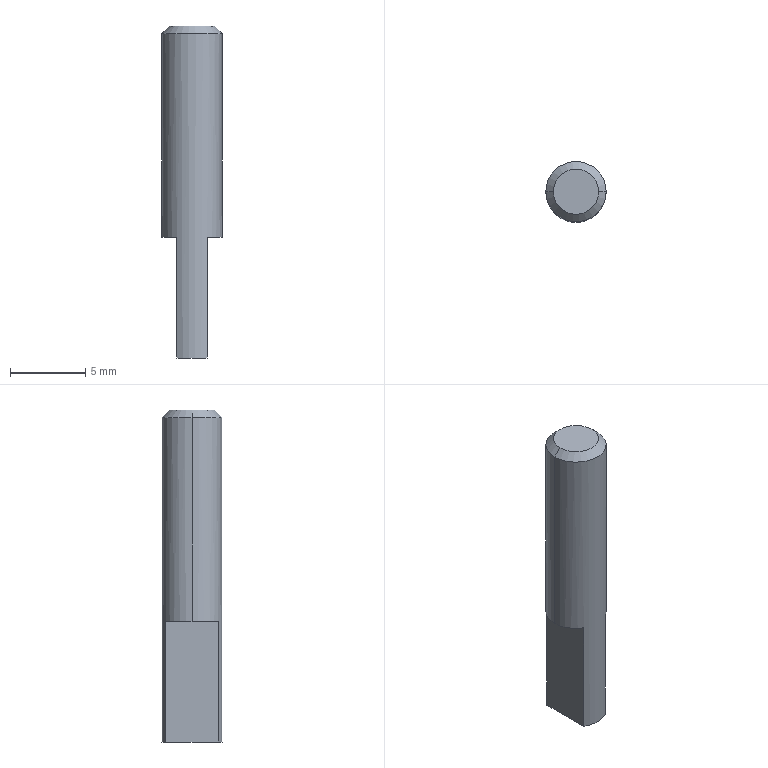Part | STEP file | PN_0104 Mount electronic clip sensor 2 | 1 solid | 10 faces | box 4 x 4 x 22 mm | volume 235.712 mm3 | plane 6 | cone 2 | cylinder 2 | commonest cylinder face diameters 4 x2
STEP:
#1=CARTESIAN_POINT('',(0.,0.,0.));
#2=DIRECTION('',(0.,0.,1.));
#3=DIRECTION('',(1.,0.,0.));
#4=AXIS2_PLACEMENT_3D('',#1,#2,#3);
#5=CARTESIAN_POINT('',(1.5,0.,22.));
#6=VERTEX_POINT('',#5);
#7=CARTESIAN_POINT('',(-1.5,0.,22.));
#8=VERTEX_POINT('',#7);
#9=CARTESIAN_POINT('',(0.,0.,22.));
#10=DIRECTION('',(0.,0.,1.));
#11=DIRECTION('',(1.,0.,0.));
#12=AXIS2_PLACEMENT_3D('',#9,#10,#11);
#13=CIRCLE('',#12,1.5);
#14=CARTESIAN_POINT('',(0.,0.,22.));
#15=DIRECTION('',(0.,0.,-1.));
#16=DIRECTION('',(-1.,0.,0.));
#17=AXIS2_PLACEMENT_3D('',#14,#15,#16);
#18=CONICAL_SURFACE('',#17,1.5,0.7854);
#19=CARTESIAN_POINT('',(3.142,0.));
#20=DIRECTION('',(-1.,0.));
#21=VECTOR('',#20,1.);
#22=LINE('',#19,#21);
#23=(GEOMETRIC_REPRESENTATION_CONTEXT(2)PARAMETRIC_REPRESENTATION_CONTEXT()REPRESENTATION_CONTEXT('',''));
#24=DEFINITIONAL_REPRESENTATION('',(#22),#23);
#25=PCURVE('',#18,#24);
#26=CARTESIAN_POINT('',(0.,0.,22.));
#27=DIRECTION('',(0.,0.,1.));
#28=DIRECTION('',(1.,0.,0.));
#29=AXIS2_PLACEMENT_3D('',#26,#27,#28);
#30=PLANE('',#29);
#31=CARTESIAN_POINT('',(0.,0.));
#32=DIRECTION('',(1.,0.));
#33=AXIS2_PLACEMENT_2D('',#31,#32);
#34=CIRCLE('',#33,1.5);
#35=(GEOMETRIC_REPRESENTATION_CONTEXT(2)PARAMETRIC_REPRESENTATION_CONTEXT()REPRESENTATION_CONTEXT('',''));
#36=DEFINITIONAL_REPRESENTATION('',(#34),#35);
#37=PCURVE('',#30,#36);
#38=SURFACE_CURVE('',#13,(#25,#37),.PCURVE_S1.);
#39=EDGE_CURVE('',#6,#8,#38,.T.);
#40=ORIENTED_EDGE('',*,*,#39,.F.);
#41=CARTESIAN_POINT('',(2.,0.,21.5));
#42=VERTEX_POINT('',#41);
#43=CARTESIAN_POINT('',(1.5,0.,22.));
#44=DIRECTION('',(0.7071,0.,-0.7071));
#45=VECTOR('',#44,1.);
#46=LINE('',#43,#45);
#47=CARTESIAN_POINT('',(3.142,0.));
#48=DIRECTION('',(0.,1.));
#49=VECTOR('',#48,1.);
#50=LINE('',#47,#49);
#51=(GEOMETRIC_REPRESENTATION_CONTEXT(2)PARAMETRIC_REPRESENTATION_CONTEXT()REPRESENTATION_CONTEXT('',''));
#52=DEFINITIONAL_REPRESENTATION('',(#50),#51);
#53=PCURVE('',#18,#52);
#54=CARTESIAN_POINT('',(0.,0.,22.));
#55=DIRECTION('',(0.,0.,-1.));
#56=DIRECTION('',(-1.,0.,0.));
#57=AXIS2_PLACEMENT_3D('',#54,#55,#56);
#58=CONICAL_SURFACE('',#57,1.5,0.7854);
#59=CARTESIAN_POINT('',(3.142,0.));
#60=DIRECTION('',(0.,1.));
#61=VECTOR('',#60,1.);
#62=LINE('',#59,#61);
#63=(GEOMETRIC_REPRESENTATION_CONTEXT(2)PARAMETRIC_REPRESENTATION_CONTEXT()REPRESENTATION_CONTEXT('',''));
#64=DEFINITIONAL_REPRESENTATION('',(#62),#63);
#65=PCURVE('',#58,#64);
#66=SURFACE_CURVE('',#46,(#53,#65),.PCURVE_S1.);
#67=EDGE_CURVE('',#6,#42,#66,.T.);
#68=ORIENTED_EDGE('',*,*,#67,.T.);
#69=CARTESIAN_POINT('',(-2.,0.,21.5));
#70=VERTEX_POINT('',#69);
#71=CARTESIAN_POINT('',(0.,0.,21.5));
#72=DIRECTION('',(0.,0.,-1.));
#73=DIRECTION('',(1.,0.,0.));
#74=AXIS2_PLACEMENT_3D('',#71,#72,#73);
#75=CIRCLE('',#74,2.);
#76=CARTESIAN_POINT('',(-3.142,0.5));
#77=DIRECTION('',(1.,0.));
#78=VECTOR('',#77,1.);
#79=LINE('',#76,#78);
#80=(GEOMETRIC_REPRESENTATION_CONTEXT(2)PARAMETRIC_REPRESENTATION_CONTEXT()REPRESENTATION_CONTEXT('',''));
#81=DEFINITIONAL_REPRESENTATION('',(#79),#80);
#82=PCURVE('',#18,#81);
#83=CARTESIAN_POINT('',(0.,0.,22.));
#84=DIRECTION('',(0.,0.,-1.));
#85=DIRECTION('',(-1.,0.,0.));
#86=AXIS2_PLACEMENT_3D('',#83,#84,#85);
#87=CYLINDRICAL_SURFACE('',#86,2.);
#88=CARTESIAN_POINT('',(-3.142,0.5));
#89=DIRECTION('',(1.,0.));
#90=VECTOR('',#89,1.);
#91=LINE('',#88,#90);
#92=(GEOMETRIC_REPRESENTATION_CONTEXT(2)PARAMETRIC_REPRESENTATION_CONTEXT()REPRESENTATION_CONTEXT('',''));
#93=DEFINITIONAL_REPRESENTATION('',(#91),#92);
#94=PCURVE('',#87,#93);
#95=SURFACE_CURVE('',#75,(#82,#94),.PCURVE_S1.);
#96=EDGE_CURVE('',#70,#42,#95,.T.);
#97=ORIENTED_EDGE('',*,*,#96,.F.);
#98=CARTESIAN_POINT('',(-1.5,0.,22.));
#99=DIRECTION('',(-0.7071,0.,-0.7071));
#100=VECTOR('',#99,1.);
#101=LINE('',#98,#100);
#102=CARTESIAN_POINT('',(0.,0.));
#103=DIRECTION('',(0.,1.));
#104=VECTOR('',#103,1.);
#105=LINE('',#102,#104);
#106=(GEOMETRIC_REPRESENTATION_CONTEXT(2)PARAMETRIC_REPRESENTATION_CONTEXT()REPRESENTATION_CONTEXT('',''));
#107=DEFINITIONAL_REPRESENTATION('',(#105),#106);
#108=PCURVE('',#18,#107);
#109=CARTESIAN_POINT('',(6.283,0.));
#110=DIRECTION('',(0.,1.));
#111=VECTOR('',#110,1.);
#112=LINE('',#109,#111);
#113=(GEOMETRIC_REPRESENTATION_CONTEXT(2)PARAMETRIC_REPRESENTATION_CONTEXT()REPRESENTATION_CONTEXT('',''));
#114=DEFINITIONAL_REPRESENTATION('',(#112),#113);
#115=PCURVE('',#58,#114);
#116=SURFACE_CURVE('',#101,(#108,#115),.PCURVE_S1.);
#117=EDGE_CURVE('',#8,#70,#116,.T.);
#118=ORIENTED_EDGE('',*,*,#117,.F.);
#119=EDGE_LOOP('',(#40,#68,#97,#118));
#120=FACE_BOUND('',#119,.T.);
#121=ADVANCED_FACE('',(#120),#18,.T.);
#122=ORIENTED_EDGE('',*,*,#96,.T.);
#123=CARTESIAN_POINT('',(2.,0.,8.));
#124=VERTEX_POINT('',#123);
#125=CARTESIAN_POINT('',(2.,0.,22.));
#126=DIRECTION('',(0.,0.,-1.));
#127=VECTOR('',#126,1.);
#128=LINE('',#125,#127);
#129=CARTESIAN_POINT('',(3.142,0.));
#130=DIRECTION('',(0.,1.));
#131=VECTOR('',#130,1.);
#132=LINE('',#129,#131);
#133=(GEOMETRIC_REPRESENTATION_CONTEXT(2)PARAMETRIC_REPRESENTATION_CONTEXT()REPRESENTATION_CONTEXT('',''));
#134=DEFINITIONAL_REPRESENTATION('',(#132),#133);
#135=PCURVE('',#87,#134);
#136=CARTESIAN_POINT('',(0.,0.,22.));
#137=DIRECTION('',(0.,0.,-1.));
#138=DIRECTION('',(-1.,0.,0.));
#139=AXIS2_PLACEMENT_3D('',#136,#137,#138);
#140=CYLINDRICAL_SURFACE('',#139,2.);
#141=CARTESIAN_POINT('',(3.142,0.));
#142=DIRECTION('',(0.,1.));
#143=VECTOR('',#142,1.);
#144=LINE('',#141,#143);
#145=(GEOMETRIC_REPRESENTATION_CONTEXT(2)PARAMETRIC_REPRESENTATION_CONTEXT()REPRESENTATION_CONTEXT('',''));
#146=DEFINITIONAL_REPRESENTATION('',(#144),#145);
#147=PCURVE('',#140,#146);
#148=SURFACE_CURVE('',#128,(#135,#147),.PCURVE_S1.);
#149=EDGE_CURVE('',#42,#124,#148,.T.);
#150=ORIENTED_EDGE('',*,*,#149,.T.);
#151=CARTESIAN_POINT('',(1.,1.732,8.));
#152=VERTEX_POINT('',#151);
#153=CARTESIAN_POINT('',(0.,0.,8.));
#154=DIRECTION('',(0.,0.,-1.));
#155=DIRECTION('',(-1.,0.,0.));
#156=AXIS2_PLACEMENT_3D('',#153,#154,#155);
#157=CIRCLE('',#156,2.);
#158=CARTESIAN_POINT('',(0.,14.));
#159=DIRECTION('',(1.,0.));
#160=VECTOR('',#159,1.);
#161=LINE('',#158,#160);
#162=(GEOMETRIC_REPRESENTATION_CONTEXT(2)PARAMETRIC_REPRESENTATION_CONTEXT()REPRESENTATION_CONTEXT('',''));
#163=DEFINITIONAL_REPRESENTATION('',(#161),#162);
#164=PCURVE('',#87,#163);
#165=CARTESIAN_POINT('',(0.,0.,8.));
#166=DIRECTION('',(0.,0.,-1.));
#167=DIRECTION('',(-1.,0.,0.));
#168=AXIS2_PLACEMENT_3D('',#165,#166,#167);
#169=PLANE('',#168);
#170=CARTESIAN_POINT('',(0.,0.));
#171=DIRECTION('',(1.,0.));
#172=AXIS2_PLACEMENT_2D('',#170,#171);
#173=CIRCLE('',#172,2.);
#174=(GEOMETRIC_REPRESENTATION_CONTEXT(2)PARAMETRIC_REPRESENTATION_CONTEXT()REPRESENTATION_CONTEXT('',''));
#175=DEFINITIONAL_REPRESENTATION('',(#173),#174);
#176=PCURVE('',#169,#175);
#177=SURFACE_CURVE('',#157,(#164,#176),.PCURVE_S1.);
#178=EDGE_CURVE('',#152,#124,#177,.T.);
#179=ORIENTED_EDGE('',*,*,#178,.F.);
#180=CARTESIAN_POINT('',(1.,1.732,0.));
#181=VERTEX_POINT('',#180);
#182=CARTESIAN_POINT('',(1.,1.732,22.));
#183=DIRECTION('',(0.,0.,-1.));
#184=VECTOR('',#183,1.);
#185=LINE('',#182,#184);
#186=CARTESIAN_POINT('',(2.094,0.));
#187=DIRECTION('',(0.,1.));
#188=VECTOR('',#187,1.);
#189=LINE('',#186,#188);
#190=(GEOMETRIC_REPRESENTATION_CONTEXT(2)PARAMETRIC_REPRESENTATION_CONTEXT()REPRESENTATION_CONTEXT('',''));
#191=DEFINITIONAL_REPRESENTATION('',(#189),#190);
#192=PCURVE('',#87,#191);
#193=CARTESIAN_POINT('',(1.,4.091,8.));
#194=DIRECTION('',(-1.,0.,0.));
#195=DIRECTION('',(0.,-1.,0.));
#196=AXIS2_PLACEMENT_3D('',#193,#194,#195);
#197=PLANE('',#196);
#198=CARTESIAN_POINT('',(2.359,14.));
#199=DIRECTION('',(0.,-1.));
#200=VECTOR('',#199,1.);
#201=LINE('',#198,#200);
#202=(GEOMETRIC_REPRESENTATION_CONTEXT(2)PARAMETRIC_REPRESENTATION_CONTEXT()REPRESENTATION_CONTEXT('',''));
#203=DEFINITIONAL_REPRESENTATION('',(#201),#202);
#204=PCURVE('',#197,#203);
#205=SURFACE_CURVE('',#185,(#192,#204),.PCURVE_S1.);
#206=EDGE_CURVE('',#152,#181,#205,.T.);
#207=ORIENTED_EDGE('',*,*,#206,.T.);
#208=CARTESIAN_POINT('',(-1.,1.732,0.));
#209=VERTEX_POINT('',#208);
#210=CARTESIAN_POINT('',(0.,0.,0.));
#211=DIRECTION('',(0.,0.,1.));
#212=DIRECTION('',(1.,0.,0.));
#213=AXIS2_PLACEMENT_3D('',#210,#211,#212);
#214=CIRCLE('',#213,2.);
#215=CARTESIAN_POINT('',(3.142,22.));
#216=DIRECTION('',(-1.,0.));
#217=VECTOR('',#216,1.);
#218=LINE('',#215,#217);
#219=(GEOMETRIC_REPRESENTATION_CONTEXT(2)PARAMETRIC_REPRESENTATION_CONTEXT()REPRESENTATION_CONTEXT('',''));
#220=DEFINITIONAL_REPRESENTATION('',(#218),#219);
#221=PCURVE('',#87,#220);
#222=CARTESIAN_POINT('',(0.,0.,0.));
#223=DIRECTION('',(0.,0.,1.));
#224=DIRECTION('',(1.,0.,0.));
#225=AXIS2_PLACEMENT_3D('',#222,#223,#224);
#226=PLANE('',#225);
#227=CARTESIAN_POINT('',(0.,0.));
#228=DIRECTION('',(1.,0.));
#229=AXIS2_PLACEMENT_2D('',#227,#228);
#230=CIRCLE('',#229,2.);
#231=(GEOMETRIC_REPRESENTATION_CONTEXT(2)PARAMETRIC_REPRESENTATION_CONTEXT()REPRESENTATION_CONTEXT('',''));
#232=DEFINITIONAL_REPRESENTATION('',(#230),#231);
#233=PCURVE('',#226,#232);
#234=SURFACE_CURVE('',#214,(#221,#233),.PCURVE_S1.);
#235=EDGE_CURVE('',#181,#209,#234,.T.);
#236=ORIENTED_EDGE('',*,*,#235,.T.);
#237=CARTESIAN_POINT('',(-1.,1.732,8.));
#238=VERTEX_POINT('',#237);
#239=CARTESIAN_POINT('',(-1.,1.732,22.));
#240=DIRECTION('',(0.,0.,1.));
#241=VECTOR('',#240,1.);
#242=LINE('',#239,#241);
#243=CARTESIAN_POINT('',(1.047,0.));
#244=DIRECTION('',(0.,-1.));
#245=VECTOR('',#244,1.);
#246=LINE('',#243,#245);
#247=(GEOMETRIC_REPRESENTATION_CONTEXT(2)PARAMETRIC_REPRESENTATION_CONTEXT()REPRESENTATION_CONTEXT('',''));
#248=DEFINITIONAL_REPRESENTATION('',(#246),#247);
#249=PCURVE('',#87,#248);
#250=CARTESIAN_POINT('',(-1.,3.929,8.));
#251=DIRECTION('',(1.,0.,0.));
#252=DIRECTION('',(0.,1.,0.));
#253=AXIS2_PLACEMENT_3D('',#250,#251,#252);
#254=PLANE('',#253);
#255=CARTESIAN_POINT('',(-2.197,14.));
#256=DIRECTION('',(0.,1.));
#257=VECTOR('',#256,1.);
#258=LINE('',#255,#257);
#259=(GEOMETRIC_REPRESENTATION_CONTEXT(2)PARAMETRIC_REPRESENTATION_CONTEXT()REPRESENTATION_CONTEXT('',''));
#260=DEFINITIONAL_REPRESENTATION('',(#258),#259);
#261=PCURVE('',#254,#260);
#262=SURFACE_CURVE('',#242,(#249,#261),.PCURVE_S1.);
#263=EDGE_CURVE('',#209,#238,#262,.T.);
#264=ORIENTED_EDGE('',*,*,#263,.T.);
#265=CARTESIAN_POINT('',(-2.,0.,8.));
#266=VERTEX_POINT('',#265);
#267=CARTESIAN_POINT('',(0.,0.,8.));
#268=DIRECTION('',(0.,0.,1.));
#269=DIRECTION('',(1.,0.,0.));
#270=AXIS2_PLACEMENT_3D('',#267,#268,#269);
#271=CIRCLE('',#270,2.);
#272=CARTESIAN_POINT('',(3.142,14.));
#273=DIRECTION('',(-1.,0.));
#274=VECTOR('',#273,1.);
#275=LINE('',#272,#274);
#276=(GEOMETRIC_REPRESENTATION_CONTEXT(2)PARAMETRIC_REPRESENTATION_CONTEXT()REPRESENTATION_CONTEXT('',''));
#277=DEFINITIONAL_REPRESENTATION('',(#275),#276);
#278=PCURVE('',#87,#277);
#279=CARTESIAN_POINT('',(0.,0.,8.));
#280=DIRECTION('',(0.,0.,1.));
#281=DIRECTION('',(1.,0.,0.));
#282=AXIS2_PLACEMENT_3D('',#279,#280,#281);
#283=PLANE('',#282);
#284=CARTESIAN_POINT('',(0.,0.));
#285=DIRECTION('',(1.,0.));
#286=AXIS2_PLACEMENT_2D('',#284,#285);
#287=CIRCLE('',#286,2.);
#288=(GEOMETRIC_REPRESENTATION_CONTEXT(2)PARAMETRIC_REPRESENTATION_CONTEXT()REPRESENTATION_CONTEXT('',''));
#289=DEFINITIONAL_REPRESENTATION('',(#287),#288);
#290=PCURVE('',#283,#289);
#291=SURFACE_CURVE('',#271,(#278,#290),.PCURVE_S1.);
#292=EDGE_CURVE('',#238,#266,#291,.T.);
#293=ORIENTED_EDGE('',*,*,#292,.T.);
#294=CARTESIAN_POINT('',(-2.,0.,22.));
#295=DIRECTION('',(0.,0.,-1.));
#296=VECTOR('',#295,1.);
#297=LINE('',#294,#296);
#298=CARTESIAN_POINT('',(0.,0.));
#299=DIRECTION('',(0.,1.));
#300=VECTOR('',#299,1.);
#301=LINE('',#298,#300);
#302=(GEOMETRIC_REPRESENTATION_CONTEXT(2)PARAMETRIC_REPRESENTATION_CONTEXT()REPRESENTATION_CONTEXT('',''));
#303=DEFINITIONAL_REPRESENTATION('',(#301),#302);
#304=PCURVE('',#87,#303);
#305=CARTESIAN_POINT('',(6.283,0.));
#306=DIRECTION('',(0.,1.));
#307=VECTOR('',#306,1.);
#308=LINE('',#305,#307);
#309=(GEOMETRIC_REPRESENTATION_CONTEXT(2)PARAMETRIC_REPRESENTATION_CONTEXT()REPRESENTATION_CONTEXT('',''));
#310=DEFINITIONAL_REPRESENTATION('',(#308),#309);
#311=PCURVE('',#140,#310);
#312=SURFACE_CURVE('',#297,(#304,#311),.PCURVE_S1.);
#313=EDGE_CURVE('',#70,#266,#312,.T.);
#314=ORIENTED_EDGE('',*,*,#313,.F.);
#315=EDGE_LOOP('',(#122,#150,#179,#207,#236,#264,#293,#314));
#316=FACE_BOUND('',#315,.T.);
#317=ADVANCED_FACE('',(#316),#87,.T.);
#318=ORIENTED_EDGE('',*,*,#149,.F.);
#319=CARTESIAN_POINT('',(0.,0.,21.5));
#320=DIRECTION('',(0.,0.,-1.));
#321=DIRECTION('',(1.,0.,0.));
#322=AXIS2_PLACEMENT_3D('',#319,#320,#321);
#323=CIRCLE('',#322,2.);
#324=CARTESIAN_POINT('',(3.142,0.5));
#325=DIRECTION('',(1.,0.));
#326=VECTOR('',#325,1.);
#327=LINE('',#324,#326);
#328=(GEOMETRIC_REPRESENTATION_CONTEXT(2)PARAMETRIC_REPRESENTATION_CONTEXT()REPRESENTATION_CONTEXT('',''));
#329=DEFINITIONAL_REPRESENTATION('',(#327),#328);
#330=PCURVE('',#140,#329);
#331=CARTESIAN_POINT('',(3.142,0.5));
#332=DIRECTION('',(1.,0.));
#333=VECTOR('',#332,1.);
#334=LINE('',#331,#333);
#335=(GEOMETRIC_REPRESENTATION_CONTEXT(2)PARAMETRIC_REPRESENTATION_CONTEXT()REPRESENTATION_CONTEXT('',''));
#336=DEFINITIONAL_REPRESENTATION('',(#334),#335);
#337=PCURVE('',#58,#336);
#338=SURFACE_CURVE('',#323,(#330,#337),.PCURVE_S1.);
#339=EDGE_CURVE('',#42,#70,#338,.T.);
#340=ORIENTED_EDGE('',*,*,#339,.T.);
#341=ORIENTED_EDGE('',*,*,#313,.T.);
#342=CARTESIAN_POINT('',(-1.,-1.732,8.));
#343=VERTEX_POINT('',#342);
#344=CARTESIAN_POINT('',(0.,0.,8.));
#345=DIRECTION('',(0.,0.,1.));
#346=DIRECTION('',(1.,0.,0.));
#347=AXIS2_PLACEMENT_3D('',#344,#345,#346);
#348=CIRCLE('',#347,2.);
#349=CARTESIAN_POINT('',(9.425,14.));
#350=DIRECTION('',(-1.,0.));
#351=VECTOR('',#350,1.);
#352=LINE('',#349,#351);
#353=(GEOMETRIC_REPRESENTATION_CONTEXT(2)PARAMETRIC_REPRESENTATION_CONTEXT()REPRESENTATION_CONTEXT('',''));
#354=DEFINITIONAL_REPRESENTATION('',(#352),#353);
#355=PCURVE('',#140,#354);
#356=CARTESIAN_POINT('',(0.,0.));
#357=DIRECTION('',(1.,0.));
#358=AXIS2_PLACEMENT_2D('',#356,#357);
#359=CIRCLE('',#358,2.);
#360=(GEOMETRIC_REPRESENTATION_CONTEXT(2)PARAMETRIC_REPRESENTATION_CONTEXT()REPRESENTATION_CONTEXT('',''));
#361=DEFINITIONAL_REPRESENTATION('',(#359),#360);
#362=PCURVE('',#283,#361);
#363=SURFACE_CURVE('',#348,(#355,#362),.PCURVE_S1.);
#364=EDGE_CURVE('',#266,#343,#363,.T.);
#365=ORIENTED_EDGE('',*,*,#364,.T.);
#366=CARTESIAN_POINT('',(-1.,-1.732,0.));
#367=VERTEX_POINT('',#366);
#368=CARTESIAN_POINT('',(-1.,-1.732,22.));
#369=DIRECTION('',(0.,0.,-1.));
#370=VECTOR('',#369,1.);
#371=LINE('',#368,#370);
#372=CARTESIAN_POINT('',(5.236,0.));
#373=DIRECTION('',(0.,1.));
#374=VECTOR('',#373,1.);
#375=LINE('',#372,#374);
#376=(GEOMETRIC_REPRESENTATION_CONTEXT(2)PARAMETRIC_REPRESENTATION_CONTEXT()REPRESENTATION_CONTEXT('',''));
#377=DEFINITIONAL_REPRESENTATION('',(#375),#376);
#378=PCURVE('',#140,#377);
#379=CARTESIAN_POINT('',(-5.661,14.));
#380=DIRECTION('',(0.,-1.));
#381=VECTOR('',#380,1.);
#382=LINE('',#379,#381);
#383=(GEOMETRIC_REPRESENTATION_CONTEXT(2)PARAMETRIC_REPRESENTATION_CONTEXT()REPRESENTATION_CONTEXT('',''));
#384=DEFINITIONAL_REPRESENTATION('',(#382),#383);
#385=PCURVE('',#254,#384);
#386=SURFACE_CURVE('',#371,(#378,#385),.PCURVE_S1.);
#387=EDGE_CURVE('',#343,#367,#386,.T.);
#388=ORIENTED_EDGE('',*,*,#387,.T.);
#389=CARTESIAN_POINT('',(1.,-1.732,0.));
#390=VERTEX_POINT('',#389);
#391=CARTESIAN_POINT('',(0.,0.,0.));
#392=DIRECTION('',(0.,0.,1.));
#393=DIRECTION('',(1.,0.,0.));
#394=AXIS2_PLACEMENT_3D('',#391,#392,#393);
#395=CIRCLE('',#394,2.);
#396=CARTESIAN_POINT('',(9.425,22.));
#397=DIRECTION('',(-1.,0.));
#398=VECTOR('',#397,1.);
#399=LINE('',#396,#398);
#400=(GEOMETRIC_REPRESENTATION_CONTEXT(2)PARAMETRIC_REPRESENTATION_CONTEXT()REPRESENTATION_CONTEXT('',''));
#401=DEFINITIONAL_REPRESENTATION('',(#399),#400);
#402=PCURVE('',#140,#401);
#403=CARTESIAN_POINT('',(0.,0.));
#404=DIRECTION('',(1.,0.));
#405=AXIS2_PLACEMENT_2D('',#403,#404);
#406=CIRCLE('',#405,2.);
#407=(GEOMETRIC_REPRESENTATION_CONTEXT(2)PARAMETRIC_REPRESENTATION_CONTEXT()REPRESENTATION_CONTEXT('',''));
#408=DEFINITIONAL_REPRESENTATION('',(#406),#407);
#409=PCURVE('',#226,#408);
#410=SURFACE_CURVE('',#395,(#402,#409),.PCURVE_S1.);
#411=EDGE_CURVE('',#367,#390,#410,.T.);
#412=ORIENTED_EDGE('',*,*,#411,.T.);
#413=CARTESIAN_POINT('',(1.,-1.732,8.));
#414=VERTEX_POINT('',#413);
#415=CARTESIAN_POINT('',(1.,-1.732,22.));
#416=DIRECTION('',(0.,0.,1.));
#417=VECTOR('',#416,1.);
#418=LINE('',#415,#417);
#419=CARTESIAN_POINT('',(4.189,0.));
#420=DIRECTION('',(0.,-1.));
#421=VECTOR('',#420,1.);
#422=LINE('',#419,#421);
#423=(GEOMETRIC_REPRESENTATION_CONTEXT(2)PARAMETRIC_REPRESENTATION_CONTEXT()REPRESENTATION_CONTEXT('',''));
#424=DEFINITIONAL_REPRESENTATION('',(#422),#423);
#425=PCURVE('',#140,#424);
#426=CARTESIAN_POINT('',(5.823,14.));
#427=DIRECTION('',(0.,1.));
#428=VECTOR('',#427,1.);
#429=LINE('',#426,#428);
#430=(GEOMETRIC_REPRESENTATION_CONTEXT(2)PARAMETRIC_REPRESENTATION_CONTEXT()REPRESENTATION_CONTEXT('',''));
#431=DEFINITIONAL_REPRESENTATION('',(#429),#430);
#432=PCURVE('',#197,#431);
#433=SURFACE_CURVE('',#418,(#425,#432),.PCURVE_S1.);
#434=EDGE_CURVE('',#390,#414,#433,.T.);
#435=ORIENTED_EDGE('',*,*,#434,.T.);
#436=CARTESIAN_POINT('',(0.,0.,8.));
#437=DIRECTION('',(0.,0.,-1.));
#438=DIRECTION('',(-1.,0.,0.));
#439=AXIS2_PLACEMENT_3D('',#436,#437,#438);
#440=CIRCLE('',#439,2.);
#441=CARTESIAN_POINT('',(0.,14.));
#442=DIRECTION('',(1.,0.));
#443=VECTOR('',#442,1.);
#444=LINE('',#441,#443);
#445=(GEOMETRIC_REPRESENTATION_CONTEXT(2)PARAMETRIC_REPRESENTATION_CONTEXT()REPRESENTATION_CONTEXT('',''));
#446=DEFINITIONAL_REPRESENTATION('',(#444),#445);
#447=PCURVE('',#140,#446);
#448=CARTESIAN_POINT('',(0.,0.));
#449=DIRECTION('',(1.,0.));
#450=AXIS2_PLACEMENT_2D('',#448,#449);
#451=CIRCLE('',#450,2.);
#452=(GEOMETRIC_REPRESENTATION_CONTEXT(2)PARAMETRIC_REPRESENTATION_CONTEXT()REPRESENTATION_CONTEXT('',''));
#453=DEFINITIONAL_REPRESENTATION('',(#451),#452);
#454=PCURVE('',#169,#453);
#455=SURFACE_CURVE('',#440,(#447,#454),.PCURVE_S1.);
#456=EDGE_CURVE('',#124,#414,#455,.T.);
#457=ORIENTED_EDGE('',*,*,#456,.F.);
#458=EDGE_LOOP('',(#318,#340,#341,#365,#388,#412,#435,#457));
#459=FACE_BOUND('',#458,.T.);
#460=ADVANCED_FACE('',(#459),#140,.T.);
#461=CARTESIAN_POINT('',(0.,0.,22.));
#462=DIRECTION('',(0.,0.,1.));
#463=DIRECTION('',(1.,0.,0.));
#464=AXIS2_PLACEMENT_3D('',#461,#462,#463);
#465=CIRCLE('',#464,1.5);
#466=CARTESIAN_POINT('',(0.,0.));
#467=DIRECTION('',(1.,0.));
#468=AXIS2_PLACEMENT_2D('',#466,#467);
#469=CIRCLE('',#468,1.5);
#470=(GEOMETRIC_REPRESENTATION_CONTEXT(2)PARAMETRIC_REPRESENTATION_CONTEXT()REPRESENTATION_CONTEXT('',''));
#471=DEFINITIONAL_REPRESENTATION('',(#469),#470);
#472=PCURVE('',#30,#471);
#473=CARTESIAN_POINT('',(9.425,0.));
#474=DIRECTION('',(-1.,0.));
#475=VECTOR('',#474,1.);
#476=LINE('',#473,#475);
#477=(GEOMETRIC_REPRESENTATION_CONTEXT(2)PARAMETRIC_REPRESENTATION_CONTEXT()REPRESENTATION_CONTEXT('',''));
#478=DEFINITIONAL_REPRESENTATION('',(#476),#477);
#479=PCURVE('',#58,#478);
#480=SURFACE_CURVE('',#465,(#472,#479),.PCURVE_S1.);
#481=EDGE_CURVE('',#8,#6,#480,.T.);
#482=ORIENTED_EDGE('',*,*,#481,.T.);
#483=ORIENTED_EDGE('',*,*,#39,.T.);
#484=EDGE_LOOP('',(#482,#483));
#485=FACE_BOUND('',#484,.T.);
#486=ADVANCED_FACE('',(#485),#30,.T.);
#487=ORIENTED_EDGE('',*,*,#411,.F.);
#488=CARTESIAN_POINT('',(-1.,0.,0.));
#489=DIRECTION('',(0.,1.,0.));
#490=VECTOR('',#489,1.);
#491=LINE('',#488,#490);
#492=CARTESIAN_POINT('',(-1.,0.));
#493=DIRECTION('',(0.,1.));
#494=VECTOR('',#493,1.);
#495=LINE('',#492,#494);
#496=(GEOMETRIC_REPRESENTATION_CONTEXT(2)PARAMETRIC_REPRESENTATION_CONTEXT()REPRESENTATION_CONTEXT('',''));
#497=DEFINITIONAL_REPRESENTATION('',(#495),#496);
#498=PCURVE('',#226,#497);
#499=CARTESIAN_POINT('',(-3.929,-8.));
#500=DIRECTION('',(1.,0.));
#501=VECTOR('',#500,1.);
#502=LINE('',#499,#501);
#503=(GEOMETRIC_REPRESENTATION_CONTEXT(2)PARAMETRIC_REPRESENTATION_CONTEXT()REPRESENTATION_CONTEXT('',''));
#504=DEFINITIONAL_REPRESENTATION('',(#502),#503);
#505=PCURVE('',#254,#504);
#506=SURFACE_CURVE('',#491,(#498,#505),.PCURVE_S1.);
#507=EDGE_CURVE('',#367,#209,#506,.T.);
#508=ORIENTED_EDGE('',*,*,#507,.T.);
#509=ORIENTED_EDGE('',*,*,#235,.F.);
#510=CARTESIAN_POINT('',(1.,0.,0.));
#511=DIRECTION('',(0.,-1.,0.));
#512=VECTOR('',#511,1.);
#513=LINE('',#510,#512);
#514=CARTESIAN_POINT('',(1.,0.));
#515=DIRECTION('',(0.,-1.));
#516=VECTOR('',#515,1.);
#517=LINE('',#514,#516);
#518=(GEOMETRIC_REPRESENTATION_CONTEXT(2)PARAMETRIC_REPRESENTATION_CONTEXT()REPRESENTATION_CONTEXT('',''));
#519=DEFINITIONAL_REPRESENTATION('',(#517),#518);
#520=PCURVE('',#226,#519);
#521=CARTESIAN_POINT('',(4.091,-8.));
#522=DIRECTION('',(1.,0.));
#523=VECTOR('',#522,1.);
#524=LINE('',#521,#523);
#525=(GEOMETRIC_REPRESENTATION_CONTEXT(2)PARAMETRIC_REPRESENTATION_CONTEXT()REPRESENTATION_CONTEXT('',''));
#526=DEFINITIONAL_REPRESENTATION('',(#524),#525);
#527=PCURVE('',#197,#526);
#528=SURFACE_CURVE('',#513,(#520,#527),.PCURVE_S1.);
#529=EDGE_CURVE('',#181,#390,#528,.T.);
#530=ORIENTED_EDGE('',*,*,#529,.T.);
#531=EDGE_LOOP('',(#487,#508,#509,#530));
#532=FACE_BOUND('',#531,.T.);
#533=ADVANCED_FACE('',(#532),#226,.F.);
#534=ORIENTED_EDGE('',*,*,#178,.T.);
#535=ORIENTED_EDGE('',*,*,#456,.T.);
#536=CARTESIAN_POINT('',(1.,4.091,8.));
#537=DIRECTION('',(0.,1.,0.));
#538=VECTOR('',#537,1.);
#539=LINE('',#536,#538);
#540=CARTESIAN_POINT('',(-1.,4.091));
#541=DIRECTION('',(0.,1.));
#542=VECTOR('',#541,1.);
#543=LINE('',#540,#542);
#544=(GEOMETRIC_REPRESENTATION_CONTEXT(2)PARAMETRIC_REPRESENTATION_CONTEXT()REPRESENTATION_CONTEXT('',''));
#545=DEFINITIONAL_REPRESENTATION('',(#543),#544);
#546=PCURVE('',#169,#545);
#547=CARTESIAN_POINT('',(0.,0.));
#548=DIRECTION('',(-1.,0.));
#549=VECTOR('',#548,1.);
#550=LINE('',#547,#549);
#551=(GEOMETRIC_REPRESENTATION_CONTEXT(2)PARAMETRIC_REPRESENTATION_CONTEXT()REPRESENTATION_CONTEXT('',''));
#552=DEFINITIONAL_REPRESENTATION('',(#550),#551);
#553=PCURVE('',#197,#552);
#554=SURFACE_CURVE('',#539,(#546,#553),.PCURVE_S1.);
#555=EDGE_CURVE('',#414,#152,#554,.T.);
#556=ORIENTED_EDGE('',*,*,#555,.T.);
#557=EDGE_LOOP('',(#534,#535,#556));
#558=FACE_BOUND('',#557,.T.);
#559=ADVANCED_FACE('',(#558),#169,.T.);
#560=ORIENTED_EDGE('',*,*,#555,.F.);
#561=ORIENTED_EDGE('',*,*,#434,.F.);
#562=ORIENTED_EDGE('',*,*,#529,.F.);
#563=ORIENTED_EDGE('',*,*,#206,.F.);
#564=EDGE_LOOP('',(#560,#561,#562,#563));
#565=FACE_BOUND('',#564,.T.);
#566=ADVANCED_FACE('',(#565),#197,.F.);
#567=CARTESIAN_POINT('',(-1.,3.929,8.));
#568=DIRECTION('',(0.,-1.,0.));
#569=VECTOR('',#568,1.);
#570=LINE('',#567,#569);
#571=CARTESIAN_POINT('',(-1.,3.929));
#572=DIRECTION('',(0.,-1.));
#573=VECTOR('',#572,1.);
#574=LINE('',#571,#573);
#575=(GEOMETRIC_REPRESENTATION_CONTEXT(2)PARAMETRIC_REPRESENTATION_CONTEXT()REPRESENTATION_CONTEXT('',''));
#576=DEFINITIONAL_REPRESENTATION('',(#574),#575);
#577=PCURVE('',#283,#576);
#578=CARTESIAN_POINT('',(0.,0.));
#579=DIRECTION('',(-1.,0.));
#580=VECTOR('',#579,1.);
#581=LINE('',#578,#580);
#582=(GEOMETRIC_REPRESENTATION_CONTEXT(2)PARAMETRIC_REPRESENTATION_CONTEXT()REPRESENTATION_CONTEXT('',''));
#583=DEFINITIONAL_REPRESENTATION('',(#581),#582);
#584=PCURVE('',#254,#583);
#585=SURFACE_CURVE('',#570,(#577,#584),.PCURVE_S1.);
#586=EDGE_CURVE('',#238,#343,#585,.T.);
#587=ORIENTED_EDGE('',*,*,#586,.T.);
#588=ORIENTED_EDGE('',*,*,#364,.F.);
#589=ORIENTED_EDGE('',*,*,#292,.F.);
#590=EDGE_LOOP('',(#587,#588,#589));
#591=FACE_BOUND('',#590,.T.);
#592=ADVANCED_FACE('',(#591),#283,.F.);
#593=ORIENTED_EDGE('',*,*,#586,.F.);
#594=ORIENTED_EDGE('',*,*,#263,.F.);
#595=ORIENTED_EDGE('',*,*,#507,.F.);
#596=ORIENTED_EDGE('',*,*,#387,.F.);
#597=EDGE_LOOP('',(#593,#594,#595,#596));
#598=FACE_BOUND('',#597,.T.);
#599=ADVANCED_FACE('',(#598),#254,.F.);
#600=ORIENTED_EDGE('',*,*,#67,.F.);
#601=ORIENTED_EDGE('',*,*,#481,.F.);
#602=ORIENTED_EDGE('',*,*,#117,.T.);
#603=ORIENTED_EDGE('',*,*,#339,.F.);
#604=EDGE_LOOP('',(#600,#601,#602,#603));
#605=FACE_BOUND('',#604,.T.);
#606=ADVANCED_FACE('',(#605),#58,.T.);
#607=CLOSED_SHELL('',(#121,#317,#460,#486,#533,#559,#566,#592,#599,#606));
#608=MANIFOLD_SOLID_BREP('',#607);
#609=(LENGTH_UNIT()NAMED_UNIT(*)SI_UNIT(.MILLI.,.METRE.));
#610=UNCERTAINTY_MEASURE_WITH_UNIT(LENGTH_MEASURE(0.0000001),#609,'','');
#611=(NAMED_UNIT(*)PLANE_ANGLE_UNIT()SI_UNIT($,.RADIAN.));
#612=(NAMED_UNIT(*)SI_UNIT($,.STERADIAN.)SOLID_ANGLE_UNIT());
#613=(GEOMETRIC_REPRESENTATION_CONTEXT(3)GLOBAL_UNCERTAINTY_ASSIGNED_CONTEXT((#610))GLOBAL_UNIT_ASSIGNED_CONTEXT((#609,#611,#612))REPRESENTATION_CONTEXT('',''));
#614=ADVANCED_BREP_SHAPE_REPRESENTATION('',(#4,#608),#613);